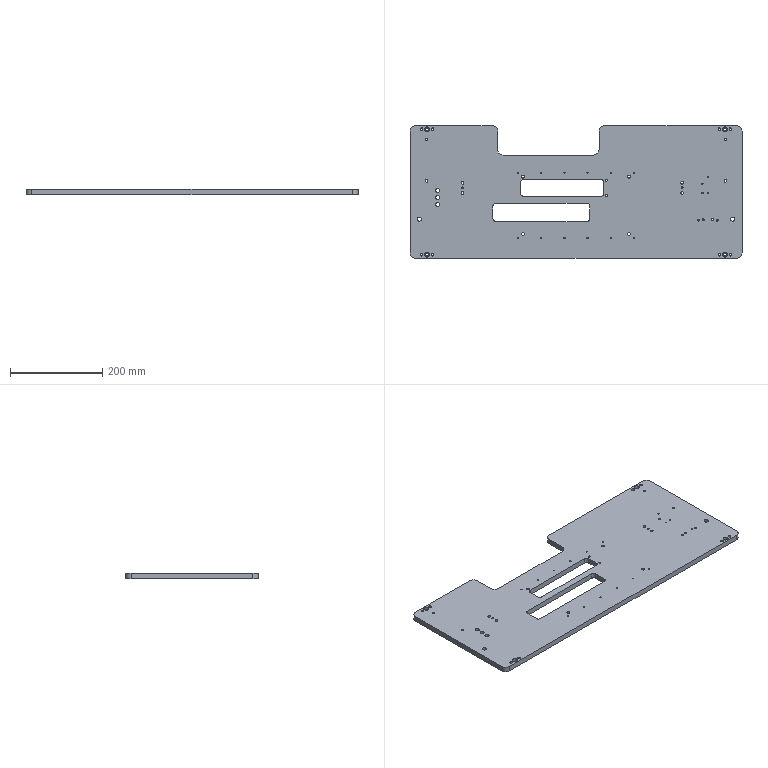Part | STEP file | QA-AD01 | 1 solid | 156 faces | box 720 x 288 x 12 mm | volume 2124409 mm3 | cylinder 130 | plane 22 | cone 4 | commonest cylinder face diameters 6 x32 2.5 x28 4.2 x12 9 x10 5 x8 6.6 x8